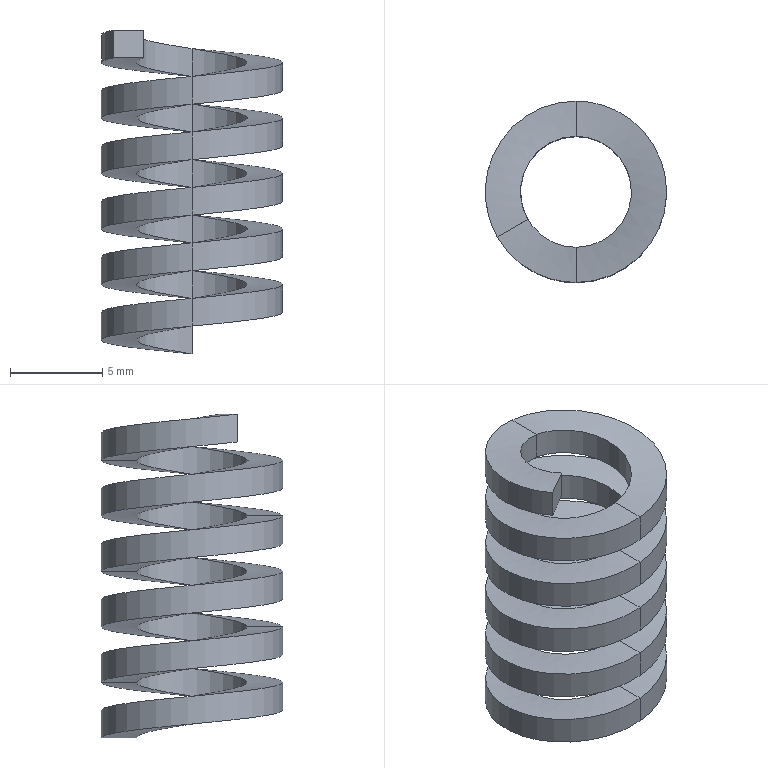Part | CATIA | 1 solid | 46 faces | box 9.8 x 9.8 x 17.5 mm | volume 377.238 mm3 | spline 44 | plane 2